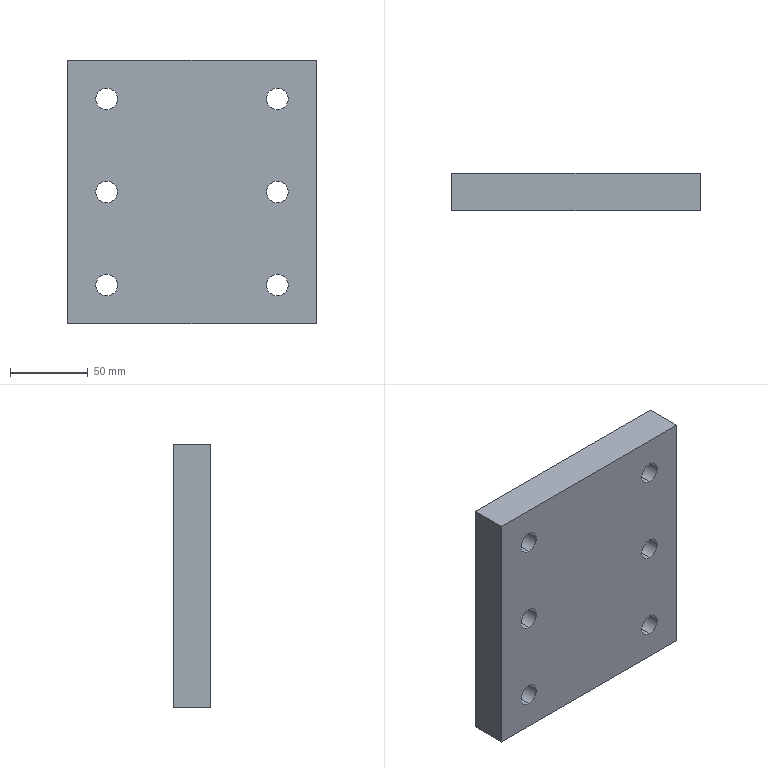Part | SolidWorks | features Extrusion 1, HoleWzd 1 | 1 solid | 18 faces | box 160 x 24 x 170 mm | volume 630633 mm3 | cylinder 12 | plane 6 | commonest cylinder face diameters 14 x12
STEP:
#1=CARTESIAN_POINT('',(-55.,0.,53.));
#2=VERTEX_POINT('',#1);
#3=CARTESIAN_POINT('',(-55.,0.,67.));
#4=VERTEX_POINT('',#3);
#5=CARTESIAN_POINT('',(-55.,0.,60.));
#6=DIRECTION('',(0.,1.,0.));
#7=DIRECTION('',(0.,0.,1.));
#8=AXIS2_PLACEMENT_3D('',#5,#6,#7);
#9=CIRCLE('',#8,7.);
#10=EDGE_CURVE('',#2,#4,#9,.T.);
#11=ORIENTED_EDGE('',*,*,#10,.F.);
#12=CARTESIAN_POINT('',(-55.,24.,53.));
#13=VERTEX_POINT('',#12);
#14=CARTESIAN_POINT('',(-55.,24.,53.));
#15=DIRECTION('',(0.,1.,0.));
#16=VECTOR('',#15,1000.);
#17=LINE('',#14,#16);
#18=EDGE_CURVE('',#2,#13,#17,.T.);
#19=ORIENTED_EDGE('',*,*,#18,.T.);
#20=CARTESIAN_POINT('',(-55.,24.,67.));
#21=VERTEX_POINT('',#20);
#22=CARTESIAN_POINT('',(-55.,24.,60.));
#23=DIRECTION('',(0.,1.,0.));
#24=DIRECTION('',(0.,0.,1.));
#25=AXIS2_PLACEMENT_3D('',#22,#23,#24);
#26=CIRCLE('',#25,7.);
#27=EDGE_CURVE('',#13,#21,#26,.T.);
#28=ORIENTED_EDGE('',*,*,#27,.T.);
#29=CARTESIAN_POINT('',(-55.,24.,67.));
#30=DIRECTION('',(0.,1.,0.));
#31=VECTOR('',#30,1000.);
#32=LINE('',#29,#31);
#33=EDGE_CURVE('',#4,#21,#32,.T.);
#34=ORIENTED_EDGE('',*,*,#33,.F.);
#35=EDGE_LOOP('',(#11,#19,#28,#34));
#36=FACE_OUTER_BOUND('',#35,.T.);
#37=CARTESIAN_POINT('',(-55.,24.,60.));
#38=DIRECTION('',(0.,1.,0.));
#39=DIRECTION('',(0.,0.,1.));
#40=AXIS2_PLACEMENT_3D('',#37,#38,#39);
#41=CYLINDRICAL_SURFACE('',#40,7.);
#42=ADVANCED_FACE('',(#36),#41,.F.);
#43=CARTESIAN_POINT('',(-55.,0.,-67.));
#44=VERTEX_POINT('',#43);
#45=CARTESIAN_POINT('',(-55.,0.,-53.));
#46=VERTEX_POINT('',#45);
#47=CARTESIAN_POINT('',(-55.,0.,-60.));
#48=DIRECTION('',(0.,1.,0.));
#49=DIRECTION('',(0.,0.,1.));
#50=AXIS2_PLACEMENT_3D('',#47,#48,#49);
#51=CIRCLE('',#50,7.);
#52=EDGE_CURVE('',#44,#46,#51,.T.);
#53=ORIENTED_EDGE('',*,*,#52,.F.);
#54=CARTESIAN_POINT('',(-55.,24.,-67.));
#55=VERTEX_POINT('',#54);
#56=CARTESIAN_POINT('',(-55.,24.,-67.));
#57=DIRECTION('',(0.,1.,0.));
#58=VECTOR('',#57,1000.);
#59=LINE('',#56,#58);
#60=EDGE_CURVE('',#44,#55,#59,.T.);
#61=ORIENTED_EDGE('',*,*,#60,.T.);
#62=CARTESIAN_POINT('',(-55.,24.,-53.));
#63=VERTEX_POINT('',#62);
#64=CARTESIAN_POINT('',(-55.,24.,-60.));
#65=DIRECTION('',(0.,1.,0.));
#66=DIRECTION('',(0.,0.,1.));
#67=AXIS2_PLACEMENT_3D('',#64,#65,#66);
#68=CIRCLE('',#67,7.);
#69=EDGE_CURVE('',#55,#63,#68,.T.);
#70=ORIENTED_EDGE('',*,*,#69,.T.);
#71=CARTESIAN_POINT('',(-55.,24.,-53.));
#72=DIRECTION('',(0.,1.,0.));
#73=VECTOR('',#72,1000.);
#74=LINE('',#71,#73);
#75=EDGE_CURVE('',#46,#63,#74,.T.);
#76=ORIENTED_EDGE('',*,*,#75,.F.);
#77=EDGE_LOOP('',(#53,#61,#70,#76));
#78=FACE_OUTER_BOUND('',#77,.T.);
#79=CARTESIAN_POINT('',(-55.,24.,-60.));
#80=DIRECTION('',(0.,1.,0.));
#81=DIRECTION('',(0.,0.,1.));
#82=AXIS2_PLACEMENT_3D('',#79,#80,#81);
#83=CYLINDRICAL_SURFACE('',#82,7.);
#84=ADVANCED_FACE('',(#78),#83,.F.);
#85=CARTESIAN_POINT('',(55.,0.,-67.));
#86=VERTEX_POINT('',#85);
#87=CARTESIAN_POINT('',(55.,0.,-53.));
#88=VERTEX_POINT('',#87);
#89=CARTESIAN_POINT('',(55.,0.,-60.));
#90=DIRECTION('',(0.,1.,0.));
#91=DIRECTION('',(0.,0.,1.));
#92=AXIS2_PLACEMENT_3D('',#89,#90,#91);
#93=CIRCLE('',#92,7.);
#94=EDGE_CURVE('',#86,#88,#93,.T.);
#95=ORIENTED_EDGE('',*,*,#94,.F.);
#96=CARTESIAN_POINT('',(55.,24.,-67.));
#97=VERTEX_POINT('',#96);
#98=CARTESIAN_POINT('',(55.,24.,-67.));
#99=DIRECTION('',(0.,1.,0.));
#100=VECTOR('',#99,1000.);
#101=LINE('',#98,#100);
#102=EDGE_CURVE('',#86,#97,#101,.T.);
#103=ORIENTED_EDGE('',*,*,#102,.T.);
#104=CARTESIAN_POINT('',(55.,24.,-53.));
#105=VERTEX_POINT('',#104);
#106=CARTESIAN_POINT('',(55.,24.,-60.));
#107=DIRECTION('',(0.,1.,0.));
#108=DIRECTION('',(0.,0.,1.));
#109=AXIS2_PLACEMENT_3D('',#106,#107,#108);
#110=CIRCLE('',#109,7.);
#111=EDGE_CURVE('',#97,#105,#110,.T.);
#112=ORIENTED_EDGE('',*,*,#111,.T.);
#113=CARTESIAN_POINT('',(55.,24.,-53.));
#114=DIRECTION('',(0.,1.,0.));
#115=VECTOR('',#114,1000.);
#116=LINE('',#113,#115);
#117=EDGE_CURVE('',#88,#105,#116,.T.);
#118=ORIENTED_EDGE('',*,*,#117,.F.);
#119=EDGE_LOOP('',(#95,#103,#112,#118));
#120=FACE_OUTER_BOUND('',#119,.T.);
#121=CARTESIAN_POINT('',(55.,24.,-60.));
#122=DIRECTION('',(0.,1.,0.));
#123=DIRECTION('',(0.,0.,1.));
#124=AXIS2_PLACEMENT_3D('',#121,#122,#123);
#125=CYLINDRICAL_SURFACE('',#124,7.);
#126=ADVANCED_FACE('',(#120),#125,.F.);
#127=CARTESIAN_POINT('',(55.,0.,53.));
#128=VERTEX_POINT('',#127);
#129=CARTESIAN_POINT('',(55.,0.,67.));
#130=VERTEX_POINT('',#129);
#131=CARTESIAN_POINT('',(55.,0.,60.));
#132=DIRECTION('',(0.,1.,0.));
#133=DIRECTION('',(0.,0.,1.));
#134=AXIS2_PLACEMENT_3D('',#131,#132,#133);
#135=CIRCLE('',#134,7.);
#136=EDGE_CURVE('',#128,#130,#135,.T.);
#137=ORIENTED_EDGE('',*,*,#136,.F.);
#138=CARTESIAN_POINT('',(55.,24.,53.));
#139=VERTEX_POINT('',#138);
#140=CARTESIAN_POINT('',(55.,24.,53.));
#141=DIRECTION('',(0.,1.,0.));
#142=VECTOR('',#141,1000.);
#143=LINE('',#140,#142);
#144=EDGE_CURVE('',#128,#139,#143,.T.);
#145=ORIENTED_EDGE('',*,*,#144,.T.);
#146=CARTESIAN_POINT('',(55.,24.,67.));
#147=VERTEX_POINT('',#146);
#148=CARTESIAN_POINT('',(55.,24.,60.));
#149=DIRECTION('',(0.,1.,0.));
#150=DIRECTION('',(0.,0.,1.));
#151=AXIS2_PLACEMENT_3D('',#148,#149,#150);
#152=CIRCLE('',#151,7.);
#153=EDGE_CURVE('',#139,#147,#152,.T.);
#154=ORIENTED_EDGE('',*,*,#153,.T.);
#155=CARTESIAN_POINT('',(55.,24.,67.));
#156=DIRECTION('',(0.,1.,0.));
#157=VECTOR('',#156,1000.);
#158=LINE('',#155,#157);
#159=EDGE_CURVE('',#130,#147,#158,.T.);
#160=ORIENTED_EDGE('',*,*,#159,.F.);
#161=EDGE_LOOP('',(#137,#145,#154,#160));
#162=FACE_OUTER_BOUND('',#161,.T.);
#163=CARTESIAN_POINT('',(55.,24.,60.));
#164=DIRECTION('',(0.,1.,0.));
#165=DIRECTION('',(0.,0.,1.));
#166=AXIS2_PLACEMENT_3D('',#163,#164,#165);
#167=CYLINDRICAL_SURFACE('',#166,7.);
#168=ADVANCED_FACE('',(#162),#167,.F.);
#169=CARTESIAN_POINT('',(55.,0.,-7.));
#170=VERTEX_POINT('',#169);
#171=CARTESIAN_POINT('',(55.,0.,7.));
#172=VERTEX_POINT('',#171);
#173=CARTESIAN_POINT('',(55.,0.,0.));
#174=DIRECTION('',(0.,1.,0.));
#175=DIRECTION('',(0.,0.,1.));
#176=AXIS2_PLACEMENT_3D('',#173,#174,#175);
#177=CIRCLE('',#176,7.);
#178=EDGE_CURVE('',#170,#172,#177,.T.);
#179=ORIENTED_EDGE('',*,*,#178,.F.);
#180=CARTESIAN_POINT('',(55.,24.,-7.));
#181=VERTEX_POINT('',#180);
#182=CARTESIAN_POINT('',(55.,24.,-7.));
#183=DIRECTION('',(0.,1.,0.));
#184=VECTOR('',#183,1000.);
#185=LINE('',#182,#184);
#186=EDGE_CURVE('',#170,#181,#185,.T.);
#187=ORIENTED_EDGE('',*,*,#186,.T.);
#188=CARTESIAN_POINT('',(55.,24.,7.));
#189=VERTEX_POINT('',#188);
#190=CARTESIAN_POINT('',(55.,24.,0.));
#191=DIRECTION('',(0.,1.,0.));
#192=DIRECTION('',(0.,0.,1.));
#193=AXIS2_PLACEMENT_3D('',#190,#191,#192);
#194=CIRCLE('',#193,7.);
#195=EDGE_CURVE('',#181,#189,#194,.T.);
#196=ORIENTED_EDGE('',*,*,#195,.T.);
#197=CARTESIAN_POINT('',(55.,24.,7.));
#198=DIRECTION('',(0.,1.,0.));
#199=VECTOR('',#198,1000.);
#200=LINE('',#197,#199);
#201=EDGE_CURVE('',#172,#189,#200,.T.);
#202=ORIENTED_EDGE('',*,*,#201,.F.);
#203=EDGE_LOOP('',(#179,#187,#196,#202));
#204=FACE_OUTER_BOUND('',#203,.T.);
#205=CARTESIAN_POINT('',(55.,24.,0.));
#206=DIRECTION('',(0.,1.,0.));
#207=DIRECTION('',(0.,0.,1.));
#208=AXIS2_PLACEMENT_3D('',#205,#206,#207);
#209=CYLINDRICAL_SURFACE('',#208,7.);
#210=ADVANCED_FACE('',(#204),#209,.F.);
#211=CARTESIAN_POINT('',(-55.,0.,-7.));
#212=VERTEX_POINT('',#211);
#213=CARTESIAN_POINT('',(-55.,0.,7.));
#214=VERTEX_POINT('',#213);
#215=CARTESIAN_POINT('',(-55.,0.,0.));
#216=DIRECTION('',(0.,1.,0.));
#217=DIRECTION('',(0.,0.,1.));
#218=AXIS2_PLACEMENT_3D('',#215,#216,#217);
#219=CIRCLE('',#218,7.);
#220=EDGE_CURVE('',#212,#214,#219,.T.);
#221=ORIENTED_EDGE('',*,*,#220,.F.);
#222=CARTESIAN_POINT('',(-55.,24.,-7.));
#223=VERTEX_POINT('',#222);
#224=CARTESIAN_POINT('',(-55.,24.,-7.));
#225=DIRECTION('',(0.,1.,0.));
#226=VECTOR('',#225,1000.);
#227=LINE('',#224,#226);
#228=EDGE_CURVE('',#212,#223,#227,.T.);
#229=ORIENTED_EDGE('',*,*,#228,.T.);
#230=CARTESIAN_POINT('',(-55.,24.,7.));
#231=VERTEX_POINT('',#230);
#232=CARTESIAN_POINT('',(-55.,24.,0.));
#233=DIRECTION('',(0.,1.,0.));
#234=DIRECTION('',(0.,0.,1.));
#235=AXIS2_PLACEMENT_3D('',#232,#233,#234);
#236=CIRCLE('',#235,7.);
#237=EDGE_CURVE('',#223,#231,#236,.T.);
#238=ORIENTED_EDGE('',*,*,#237,.T.);
#239=CARTESIAN_POINT('',(-55.,24.,7.));
#240=DIRECTION('',(0.,1.,0.));
#241=VECTOR('',#240,1000.);
#242=LINE('',#239,#241);
#243=EDGE_CURVE('',#214,#231,#242,.T.);
#244=ORIENTED_EDGE('',*,*,#243,.F.);
#245=EDGE_LOOP('',(#221,#229,#238,#244));
#246=FACE_OUTER_BOUND('',#245,.T.);
#247=CARTESIAN_POINT('',(-55.,24.,0.));
#248=DIRECTION('',(0.,1.,0.));
#249=DIRECTION('',(0.,0.,1.));
#250=AXIS2_PLACEMENT_3D('',#247,#248,#249);
#251=CYLINDRICAL_SURFACE('',#250,7.);
#252=ADVANCED_FACE('',(#246),#251,.F.);
#253=CARTESIAN_POINT('',(80.,0.,85.));
#254=VERTEX_POINT('',#253);
#255=CARTESIAN_POINT('',(80.,0.,-85.));
#256=VERTEX_POINT('',#255);
#257=CARTESIAN_POINT('',(80.,0.,85.));
#258=DIRECTION('',(0.,0.,-1.));
#259=VECTOR('',#258,1000.);
#260=LINE('',#257,#259);
#261=EDGE_CURVE('',#254,#256,#260,.T.);
#262=ORIENTED_EDGE('',*,*,#261,.T.);
#263=CARTESIAN_POINT('',(80.,24.,-85.));
#264=VERTEX_POINT('',#263);
#265=CARTESIAN_POINT('',(80.,24.,-85.));
#266=DIRECTION('',(0.,-1.,0.));
#267=VECTOR('',#266,1000.);
#268=LINE('',#265,#267);
#269=EDGE_CURVE('',#264,#256,#268,.T.);
#270=ORIENTED_EDGE('',*,*,#269,.F.);
#271=CARTESIAN_POINT('',(80.,24.,85.));
#272=VERTEX_POINT('',#271);
#273=CARTESIAN_POINT('',(80.,24.,85.));
#274=DIRECTION('',(0.,0.,-1.));
#275=VECTOR('',#274,1000.);
#276=LINE('',#273,#275);
#277=EDGE_CURVE('',#272,#264,#276,.T.);
#278=ORIENTED_EDGE('',*,*,#277,.F.);
#279=CARTESIAN_POINT('',(80.,24.,85.));
#280=DIRECTION('',(0.,-1.,0.));
#281=VECTOR('',#280,1000.);
#282=LINE('',#279,#281);
#283=EDGE_CURVE('',#272,#254,#282,.T.);
#284=ORIENTED_EDGE('',*,*,#283,.T.);
#285=EDGE_LOOP('',(#262,#270,#278,#284));
#286=FACE_OUTER_BOUND('',#285,.T.);
#287=CARTESIAN_POINT('',(80.,24.,85.));
#288=DIRECTION('',(-1.,0.,0.));
#289=DIRECTION('',(0.,0.,1.));
#290=AXIS2_PLACEMENT_3D('',#287,#288,#289);
#291=PLANE('',#290);
#292=ADVANCED_FACE('',(#286),#291,.F.);
#293=CARTESIAN_POINT('',(-80.,0.,-85.));
#294=VERTEX_POINT('',#293);
#295=CARTESIAN_POINT('',(-80.,0.,-85.));
#296=DIRECTION('',(-1.,0.,0.));
#297=VECTOR('',#296,1000.);
#298=LINE('',#295,#297);
#299=EDGE_CURVE('',#256,#294,#298,.T.);
#300=ORIENTED_EDGE('',*,*,#299,.T.);
#301=CARTESIAN_POINT('',(-80.,24.,-85.));
#302=VERTEX_POINT('',#301);
#303=CARTESIAN_POINT('',(-80.,24.,-85.));
#304=DIRECTION('',(0.,-1.,0.));
#305=VECTOR('',#304,1000.);
#306=LINE('',#303,#305);
#307=EDGE_CURVE('',#302,#294,#306,.T.);
#308=ORIENTED_EDGE('',*,*,#307,.F.);
#309=CARTESIAN_POINT('',(-80.,24.,-85.));
#310=DIRECTION('',(-1.,0.,0.));
#311=VECTOR('',#310,1000.);
#312=LINE('',#309,#311);
#313=EDGE_CURVE('',#264,#302,#312,.T.);
#314=ORIENTED_EDGE('',*,*,#313,.F.);
#315=ORIENTED_EDGE('',*,*,#269,.T.);
#316=EDGE_LOOP('',(#300,#308,#314,#315));
#317=FACE_OUTER_BOUND('',#316,.T.);
#318=CARTESIAN_POINT('',(-80.,24.,-85.));
#319=DIRECTION('',(0.,0.,1.));
#320=DIRECTION('',(1.,0.,0.));
#321=AXIS2_PLACEMENT_3D('',#318,#319,#320);
#322=PLANE('',#321);
#323=ADVANCED_FACE('',(#317),#322,.F.);
#324=CARTESIAN_POINT('',(-80.,0.,85.));
#325=VERTEX_POINT('',#324);
#326=CARTESIAN_POINT('',(-80.,0.,85.));
#327=DIRECTION('',(0.,0.,1.));
#328=VECTOR('',#327,1000.);
#329=LINE('',#326,#328);
#330=EDGE_CURVE('',#294,#325,#329,.T.);
#331=ORIENTED_EDGE('',*,*,#330,.T.);
#332=CARTESIAN_POINT('',(-80.,24.,85.));
#333=VERTEX_POINT('',#332);
#334=CARTESIAN_POINT('',(-80.,24.,85.));
#335=DIRECTION('',(0.,-1.,0.));
#336=VECTOR('',#335,1000.);
#337=LINE('',#334,#336);
#338=EDGE_CURVE('',#333,#325,#337,.T.);
#339=ORIENTED_EDGE('',*,*,#338,.F.);
#340=CARTESIAN_POINT('',(-80.,24.,85.));
#341=DIRECTION('',(0.,0.,1.));
#342=VECTOR('',#341,1000.);
#343=LINE('',#340,#342);
#344=EDGE_CURVE('',#302,#333,#343,.T.);
#345=ORIENTED_EDGE('',*,*,#344,.F.);
#346=ORIENTED_EDGE('',*,*,#307,.T.);
#347=EDGE_LOOP('',(#331,#339,#345,#346));
#348=FACE_OUTER_BOUND('',#347,.T.);
#349=CARTESIAN_POINT('',(-80.,24.,85.));
#350=DIRECTION('',(1.,0.,0.));
#351=DIRECTION('',(0.,0.,-1.));
#352=AXIS2_PLACEMENT_3D('',#349,#350,#351);
#353=PLANE('',#352);
#354=ADVANCED_FACE('',(#348),#353,.F.);
#355=CARTESIAN_POINT('',(-80.,0.,85.));
#356=DIRECTION('',(1.,0.,0.));
#357=VECTOR('',#356,1000.);
#358=LINE('',#355,#357);
#359=EDGE_CURVE('',#325,#254,#358,.T.);
#360=ORIENTED_EDGE('',*,*,#359,.T.);
#361=ORIENTED_EDGE('',*,*,#283,.F.);
#362=CARTESIAN_POINT('',(-80.,24.,85.));
#363=DIRECTION('',(1.,0.,0.));
#364=VECTOR('',#363,1000.);
#365=LINE('',#362,#364);
#366=EDGE_CURVE('',#333,#272,#365,.T.);
#367=ORIENTED_EDGE('',*,*,#366,.F.);
#368=ORIENTED_EDGE('',*,*,#338,.T.);
#369=EDGE_LOOP('',(#360,#361,#367,#368));
#370=FACE_OUTER_BOUND('',#369,.T.);
#371=CARTESIAN_POINT('',(-80.,24.,85.));
#372=DIRECTION('',(0.,0.,-1.));
#373=DIRECTION('',(-1.,0.,0.));
#374=AXIS2_PLACEMENT_3D('',#371,#372,#373);
#375=PLANE('',#374);
#376=ADVANCED_FACE('',(#370),#375,.F.);
#377=CARTESIAN_POINT('',(-55.,24.,60.));
#378=DIRECTION('',(0.,1.,0.));
#379=DIRECTION('',(0.,0.,1.));
#380=AXIS2_PLACEMENT_3D('',#377,#378,#379);
#381=CIRCLE('',#380,7.);
#382=EDGE_CURVE('',#21,#13,#381,.T.);
#383=ORIENTED_EDGE('',*,*,#382,.F.);
#384=ORIENTED_EDGE('',*,*,#27,.F.);
#385=EDGE_LOOP('',(#383,#384));
#386=FACE_BOUND('',#385,.T.);
#387=CARTESIAN_POINT('',(-55.,24.,-60.));
#388=DIRECTION('',(0.,1.,0.));
#389=DIRECTION('',(0.,0.,1.));
#390=AXIS2_PLACEMENT_3D('',#387,#388,#389);
#391=CIRCLE('',#390,7.);
#392=EDGE_CURVE('',#63,#55,#391,.T.);
#393=ORIENTED_EDGE('',*,*,#392,.F.);
#394=ORIENTED_EDGE('',*,*,#69,.F.);
#395=EDGE_LOOP('',(#393,#394));
#396=FACE_BOUND('',#395,.T.);
#397=CARTESIAN_POINT('',(55.,24.,-60.));
#398=DIRECTION('',(0.,1.,0.));
#399=DIRECTION('',(0.,0.,1.));
#400=AXIS2_PLACEMENT_3D('',#397,#398,#399);
#401=CIRCLE('',#400,7.);
#402=EDGE_CURVE('',#105,#97,#401,.T.);
#403=ORIENTED_EDGE('',*,*,#402,.F.);
#404=ORIENTED_EDGE('',*,*,#111,.F.);
#405=EDGE_LOOP('',(#403,#404));
#406=FACE_BOUND('',#405,.T.);
#407=CARTESIAN_POINT('',(55.,24.,60.));
#408=DIRECTION('',(0.,1.,0.));
#409=DIRECTION('',(0.,0.,1.));
#410=AXIS2_PLACEMENT_3D('',#407,#408,#409);
#411=CIRCLE('',#410,7.);
#412=EDGE_CURVE('',#147,#139,#411,.T.);
#413=ORIENTED_EDGE('',*,*,#412,.F.);
#414=ORIENTED_EDGE('',*,*,#153,.F.);
#415=EDGE_LOOP('',(#413,#414));
#416=FACE_BOUND('',#415,.T.);
#417=CARTESIAN_POINT('',(55.,24.,0.));
#418=DIRECTION('',(0.,1.,0.));
#419=DIRECTION('',(0.,0.,1.));
#420=AXIS2_PLACEMENT_3D('',#417,#418,#419);
#421=CIRCLE('',#420,7.);
#422=EDGE_CURVE('',#189,#181,#421,.T.);
#423=ORIENTED_EDGE('',*,*,#422,.F.);
#424=ORIENTED_EDGE('',*,*,#195,.F.);
#425=EDGE_LOOP('',(#423,#424));
#426=FACE_BOUND('',#425,.T.);
#427=CARTESIAN_POINT('',(-55.,24.,0.));
#428=DIRECTION('',(0.,1.,0.));
#429=DIRECTION('',(0.,0.,1.));
#430=AXIS2_PLACEMENT_3D('',#427,#428,#429);
#431=CIRCLE('',#430,7.);
#432=EDGE_CURVE('',#231,#223,#431,.T.);
#433=ORIENTED_EDGE('',*,*,#432,.F.);
#434=ORIENTED_EDGE('',*,*,#237,.F.);
#435=EDGE_LOOP('',(#433,#434));
#436=FACE_BOUND('',#435,.T.);
#437=ORIENTED_EDGE('',*,*,#277,.T.);
#438=ORIENTED_EDGE('',*,*,#313,.T.);
#439=ORIENTED_EDGE('',*,*,#344,.T.);
#440=ORIENTED_EDGE('',*,*,#366,.T.);
#441=EDGE_LOOP('',(#437,#438,#439,#440));
#442=FACE_OUTER_BOUND('',#441,.T.);
#443=CARTESIAN_POINT('',(0.,24.,0.));
#444=DIRECTION('',(0.,-1.,0.));
#445=DIRECTION('',(0.,0.,-1.));
#446=AXIS2_PLACEMENT_3D('',#443,#444,#445);
#447=PLANE('',#446);
#448=ADVANCED_FACE('',(#386,#396,#406,#416,#426,#436,#442),#447,.F.);
#449=CARTESIAN_POINT('',(-55.,0.,60.));
#450=DIRECTION('',(0.,1.,0.));
#451=DIRECTION('',(0.,0.,1.));
#452=AXIS2_PLACEMENT_3D('',#449,#450,#451);
#453=CIRCLE('',#452,7.);
#454=EDGE_CURVE('',#4,#2,#453,.T.);
#455=ORIENTED_EDGE('',*,*,#454,.T.);
#456=ORIENTED_EDGE('',*,*,#10,.T.);
#457=EDGE_LOOP('',(#455,#456));
#458=FACE_BOUND('',#457,.T.);
#459=CARTESIAN_POINT('',(-55.,0.,-60.));
#460=DIRECTION('',(0.,1.,0.));
#461=DIRECTION('',(0.,0.,1.));
#462=AXIS2_PLACEMENT_3D('',#459,#460,#461);
#463=CIRCLE('',#462,7.);
#464=EDGE_CURVE('',#46,#44,#463,.T.);
#465=ORIENTED_EDGE('',*,*,#464,.T.);
#466=ORIENTED_EDGE('',*,*,#52,.T.);
#467=EDGE_LOOP('',(#465,#466));
#468=FACE_BOUND('',#467,.T.);
#469=CARTESIAN_POINT('',(55.,0.,-60.));
#470=DIRECTION('',(0.,1.,0.));
#471=DIRECTION('',(0.,0.,1.));
#472=AXIS2_PLACEMENT_3D('',#469,#470,#471);
#473=CIRCLE('',#472,7.);
#474=EDGE_CURVE('',#88,#86,#473,.T.);
#475=ORIENTED_EDGE('',*,*,#474,.T.);
#476=ORIENTED_EDGE('',*,*,#94,.T.);
#477=EDGE_LOOP('',(#475,#476));
#478=FACE_BOUND('',#477,.T.);
#479=CARTESIAN_POINT('',(55.,0.,60.));
#480=DIRECTION('',(0.,1.,0.));
#481=DIRECTION('',(0.,0.,1.));
#482=AXIS2_PLACEMENT_3D('',#479,#480,#481);
#483=CIRCLE('',#482,7.);
#484=EDGE_CURVE('',#130,#128,#483,.T.);
#485=ORIENTED_EDGE('',*,*,#484,.T.);
#486=ORIENTED_EDGE('',*,*,#136,.T.);
#487=EDGE_LOOP('',(#485,#486));
#488=FACE_BOUND('',#487,.T.);
#489=CARTESIAN_POINT('',(55.,0.,0.));
#490=DIRECTION('',(0.,1.,0.));
#491=DIRECTION('',(0.,0.,1.));
#492=AXIS2_PLACEMENT_3D('',#489,#490,#491);
#493=CIRCLE('',#492,7.);
#494=EDGE_CURVE('',#172,#170,#493,.T.);
#495=ORIENTED_EDGE('',*,*,#494,.T.);
#496=ORIENTED_EDGE('',*,*,#178,.T.);
#497=EDGE_LOOP('',(#495,#496));
#498=FACE_BOUND('',#497,.T.);
#499=CARTESIAN_POINT('',(-55.,0.,0.));
#500=DIRECTION('',(0.,1.,0.));
#501=DIRECTION('',(0.,0.,1.));
#502=AXIS2_PLACEMENT_3D('',#499,#500,#501);
#503=CIRCLE('',#502,7.);
#504=EDGE_CURVE('',#214,#212,#503,.T.);
#505=ORIENTED_EDGE('',*,*,#504,.T.);
#506=ORIENTED_EDGE('',*,*,#220,.T.);
#507=EDGE_LOOP('',(#505,#506));
#508=FACE_BOUND('',#507,.T.);
#509=ORIENTED_EDGE('',*,*,#261,.F.);
#510=ORIENTED_EDGE('',*,*,#359,.F.);
#511=ORIENTED_EDGE('',*,*,#330,.F.);
#512=ORIENTED_EDGE('',*,*,#299,.F.);
#513=EDGE_LOOP('',(#509,#510,#511,#512));
#514=FACE_OUTER_BOUND('',#513,.T.);
#515=CARTESIAN_POINT('',(0.,0.,0.));
#516=DIRECTION('',(0.,-1.,0.));
#517=DIRECTION('',(0.,0.,-1.));
#518=AXIS2_PLACEMENT_3D('',#515,#516,#517);
#519=PLANE('',#518);
#520=ADVANCED_FACE('',(#458,#468,#478,#488,#498,#508,#514),#519,.T.);
#521=ORIENTED_EDGE('',*,*,#228,.F.);
#522=ORIENTED_EDGE('',*,*,#504,.F.);
#523=ORIENTED_EDGE('',*,*,#243,.T.);
#524=ORIENTED_EDGE('',*,*,#432,.T.);
#525=EDGE_LOOP('',(#521,#522,#523,#524));
#526=FACE_OUTER_BOUND('',#525,.T.);
#527=CARTESIAN_POINT('',(-55.,24.,0.));
#528=DIRECTION('',(0.,1.,0.));
#529=DIRECTION('',(0.,0.,1.));
#530=AXIS2_PLACEMENT_3D('',#527,#528,#529);
#531=CYLINDRICAL_SURFACE('',#530,7.);
#532=ADVANCED_FACE('',(#526),#531,.F.);
#533=ORIENTED_EDGE('',*,*,#186,.F.);
#534=ORIENTED_EDGE('',*,*,#494,.F.);
#535=ORIENTED_EDGE('',*,*,#201,.T.);
#536=ORIENTED_EDGE('',*,*,#422,.T.);
#537=EDGE_LOOP('',(#533,#534,#535,#536));
#538=FACE_OUTER_BOUND('',#537,.T.);
#539=CARTESIAN_POINT('',(55.,24.,0.));
#540=DIRECTION('',(0.,1.,0.));
#541=DIRECTION('',(0.,0.,1.));
#542=AXIS2_PLACEMENT_3D('',#539,#540,#541);
#543=CYLINDRICAL_SURFACE('',#542,7.);
#544=ADVANCED_FACE('',(#538),#543,.F.);
#545=ORIENTED_EDGE('',*,*,#144,.F.);
#546=ORIENTED_EDGE('',*,*,#484,.F.);
#547=ORIENTED_EDGE('',*,*,#159,.T.);
#548=ORIENTED_EDGE('',*,*,#412,.T.);
#549=EDGE_LOOP('',(#545,#546,#547,#548));
#550=FACE_OUTER_BOUND('',#549,.T.);
#551=CARTESIAN_POINT('',(55.,24.,60.));
#552=DIRECTION('',(0.,1.,0.));
#553=DIRECTION('',(0.,0.,1.));
#554=AXIS2_PLACEMENT_3D('',#551,#552,#553);
#555=CYLINDRICAL_SURFACE('',#554,7.);
#556=ADVANCED_FACE('',(#550),#555,.F.);
#557=ORIENTED_EDGE('',*,*,#102,.F.);
#558=ORIENTED_EDGE('',*,*,#474,.F.);
#559=ORIENTED_EDGE('',*,*,#117,.T.);
#560=ORIENTED_EDGE('',*,*,#402,.T.);
#561=EDGE_LOOP('',(#557,#558,#559,#560));
#562=FACE_OUTER_BOUND('',#561,.T.);
#563=CARTESIAN_POINT('',(55.,24.,-60.));
#564=DIRECTION('',(0.,1.,0.));
#565=DIRECTION('',(0.,0.,1.));
#566=AXIS2_PLACEMENT_3D('',#563,#564,#565);
#567=CYLINDRICAL_SURFACE('',#566,7.);
#568=ADVANCED_FACE('',(#562),#567,.F.);
#569=ORIENTED_EDGE('',*,*,#60,.F.);
#570=ORIENTED_EDGE('',*,*,#464,.F.);
#571=ORIENTED_EDGE('',*,*,#75,.T.);
#572=ORIENTED_EDGE('',*,*,#392,.T.);
#573=EDGE_LOOP('',(#569,#570,#571,#572));
#574=FACE_OUTER_BOUND('',#573,.T.);
#575=CARTESIAN_POINT('',(-55.,24.,-60.));
#576=DIRECTION('',(0.,1.,0.));
#577=DIRECTION('',(0.,0.,1.));
#578=AXIS2_PLACEMENT_3D('',#575,#576,#577);
#579=CYLINDRICAL_SURFACE('',#578,7.);
#580=ADVANCED_FACE('',(#574),#579,.F.);
#581=ORIENTED_EDGE('',*,*,#18,.F.);
#582=ORIENTED_EDGE('',*,*,#454,.F.);
#583=ORIENTED_EDGE('',*,*,#33,.T.);
#584=ORIENTED_EDGE('',*,*,#382,.T.);
#585=EDGE_LOOP('',(#581,#582,#583,#584));
#586=FACE_OUTER_BOUND('',#585,.T.);
#587=CARTESIAN_POINT('',(-55.,24.,60.));
#588=DIRECTION('',(0.,1.,0.));
#589=DIRECTION('',(0.,0.,1.));
#590=AXIS2_PLACEMENT_3D('',#587,#588,#589);
#591=CYLINDRICAL_SURFACE('',#590,7.);
#592=ADVANCED_FACE('',(#586),#591,.F.);
#593=CLOSED_SHELL('',(#42,#84,#126,#168,#210,#252,#292,#323,#354,#376,#448,#520,#532,#544,#556,#568,#580,#592));
#594=MANIFOLD_SOLID_BREP('',#593);
#595=CARTESIAN_POINT('',(0.,0.,0.));
#596=DIRECTION('',(0.,0.,1.));
#597=DIRECTION('',(1.,0.,0.));
#598=AXIS2_PLACEMENT_3D('',#595,#596,#597);
#599=(LENGTH_UNIT()NAMED_UNIT(*)SI_UNIT(.MILLI.,.METRE.));
#600=UNCERTAINTY_MEASURE_WITH_UNIT(LENGTH_MEASURE(0.00001),#599,'','');
#601=(NAMED_UNIT(*)PLANE_ANGLE_UNIT()SI_UNIT($,.RADIAN.));
#602=(NAMED_UNIT(*)SI_UNIT($,.STERADIAN.)SOLID_ANGLE_UNIT());
#603=(GEOMETRIC_REPRESENTATION_CONTEXT(3)GLOBAL_UNCERTAINTY_ASSIGNED_CONTEXT((#600))GLOBAL_UNIT_ASSIGNED_CONTEXT((#599,#601,#602))REPRESENTATION_CONTEXT('',''));
#604=ADVANCED_BREP_SHAPE_REPRESENTATION('',(#594,#598),#603);